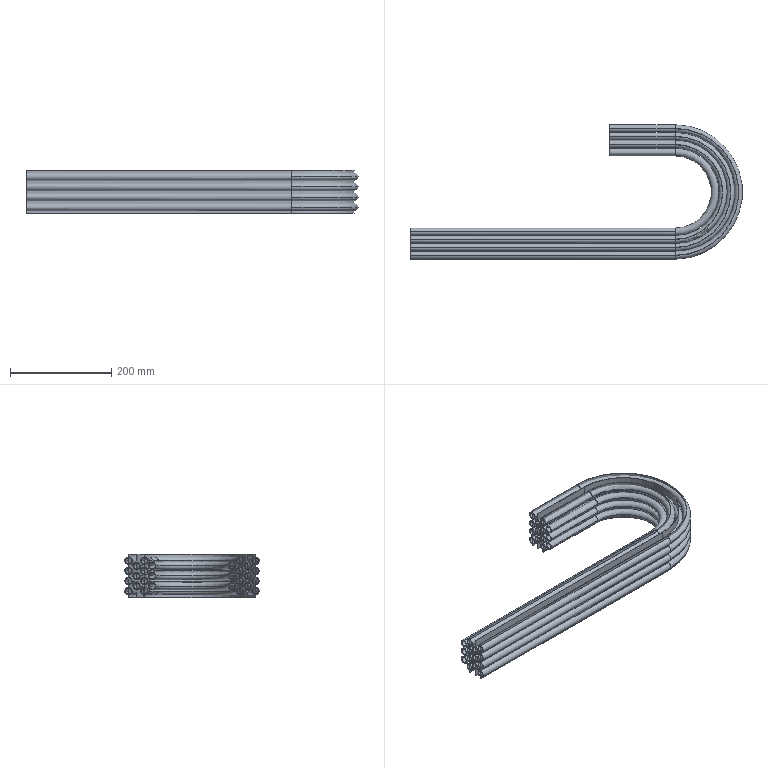Part | STEP file | 14 solids | 282 faces | box 658 x 266 x 85.182 mm | volume 995637 mm3 | cylinder 134 | plane 80 | torus 62 | cone 6 | commonest cylinder face diameters 12 x59 15 x59 219.5 x7 220.5 x7 250.5 x1 251.5 x1